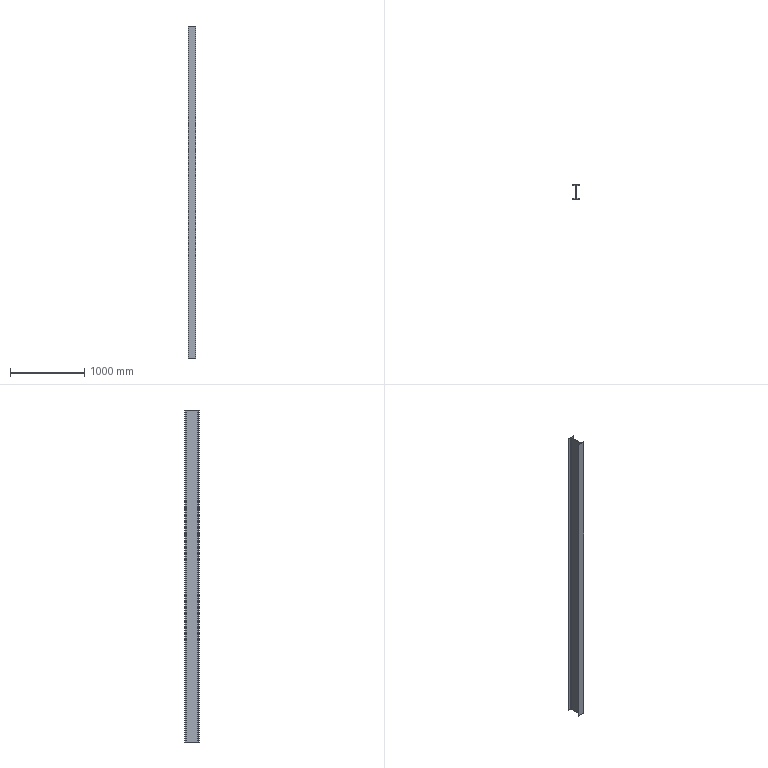Part | SolidWorks | features Extrusion 1, MoveFace 1 | 1 solid | 18 faces | box 100 x 200 x 4480 mm | volume 12833917 mm3 | plane 10 | cylinder 8 | commonest cylinder face diameters 9 x4 18 x4
STEP:
#1=CARTESIAN_POINT('',(314.405,123.017,-900.));
#2=VERTEX_POINT('',#1);
#3=CARTESIAN_POINT('',(321.925,131.894,-900.));
#4=VERTEX_POINT('',#3);
#5=CARTESIAN_POINT('',(323.405,123.017,-900.));
#6=DIRECTION('',(0.,0.,-1.));
#7=DIRECTION('',(1.,0.,0.));
#8=AXIS2_PLACEMENT_3D('',#5,#6,#7);
#9=CIRCLE('',#8,9.);
#10=EDGE_CURVE('',#2,#4,#9,.T.);
#11=ORIENTED_EDGE('',*,*,#10,.T.);
#12=CARTESIAN_POINT('',(321.925,131.894,3580.));
#13=VERTEX_POINT('',#12);
#14=CARTESIAN_POINT('',(321.925,131.894,3580.));
#15=DIRECTION('',(0.,0.,-1.));
#16=VECTOR('',#15,1000.);
#17=LINE('',#14,#16);
#18=EDGE_CURVE('',#13,#4,#17,.T.);
#19=ORIENTED_EDGE('',*,*,#18,.F.);
#20=CARTESIAN_POINT('',(314.405,123.017,3580.));
#21=VERTEX_POINT('',#20);
#22=CARTESIAN_POINT('',(323.405,123.017,3580.));
#23=DIRECTION('',(0.,0.,-1.));
#24=DIRECTION('',(1.,0.,0.));
#25=AXIS2_PLACEMENT_3D('',#22,#23,#24);
#26=CIRCLE('',#25,9.);
#27=EDGE_CURVE('',#21,#13,#26,.T.);
#28=ORIENTED_EDGE('',*,*,#27,.F.);
#29=CARTESIAN_POINT('',(314.405,123.017,3580.));
#30=DIRECTION('',(0.,0.,-1.));
#31=VECTOR('',#30,1000.);
#32=LINE('',#29,#31);
#33=EDGE_CURVE('',#21,#2,#32,.T.);
#34=ORIENTED_EDGE('',*,*,#33,.T.);
#35=EDGE_LOOP('',(#11,#19,#28,#34));
#36=FACE_OUTER_BOUND('',#35,.T.);
#37=CARTESIAN_POINT('',(323.405,123.017,3580.));
#38=DIRECTION('',(0.,0.,-1.));
#39=DIRECTION('',(-1.,0.,0.));
#40=AXIS2_PLACEMENT_3D('',#37,#38,#39);
#41=CYLINDRICAL_SURFACE('',#40,9.);
#42=ADVANCED_FACE('',(#36),#41,.F.);
#43=CARTESIAN_POINT('',(357.144,137.763,-900.));
#44=VERTEX_POINT('',#43);
#45=CARTESIAN_POINT('',(321.925,131.894,-900.));
#46=DIRECTION('',(0.9864,0.1644,0.));
#47=VECTOR('',#46,1000.);
#48=LINE('',#45,#47);
#49=EDGE_CURVE('',#4,#44,#48,.T.);
#50=ORIENTED_EDGE('',*,*,#49,.T.);
#51=CARTESIAN_POINT('',(357.144,137.763,3580.));
#52=VERTEX_POINT('',#51);
#53=CARTESIAN_POINT('',(357.144,137.763,3580.));
#54=DIRECTION('',(0.,0.,-1.));
#55=VECTOR('',#54,1000.);
#56=LINE('',#53,#55);
#57=EDGE_CURVE('',#52,#44,#56,.T.);
#58=ORIENTED_EDGE('',*,*,#57,.F.);
#59=CARTESIAN_POINT('',(321.925,131.894,3580.));
#60=DIRECTION('',(0.9864,0.1644,0.));
#61=VECTOR('',#60,1000.);
#62=LINE('',#59,#61);
#63=EDGE_CURVE('',#13,#52,#62,.T.);
#64=ORIENTED_EDGE('',*,*,#63,.F.);
#65=ORIENTED_EDGE('',*,*,#18,.T.);
#66=EDGE_LOOP('',(#50,#58,#64,#65));
#67=FACE_OUTER_BOUND('',#66,.T.);
#68=CARTESIAN_POINT('',(321.925,131.894,3580.));
#69=DIRECTION('',(-0.1644,0.9864,0.));
#70=DIRECTION('',(-0.9864,-0.1644,0.));
#71=AXIS2_PLACEMENT_3D('',#68,#69,#70);
#72=PLANE('',#71);
#73=ADVANCED_FACE('',(#67),#72,.F.);
#74=CARTESIAN_POINT('',(360.905,142.202,-900.));
#75=VERTEX_POINT('',#74);
#76=CARTESIAN_POINT('',(356.405,142.202,-900.));
#77=DIRECTION('',(0.,0.,1.));
#78=DIRECTION('',(1.,0.,0.));
#79=AXIS2_PLACEMENT_3D('',#76,#77,#78);
#80=CIRCLE('',#79,4.5);
#81=EDGE_CURVE('',#44,#75,#80,.T.);
#82=ORIENTED_EDGE('',*,*,#81,.T.);
#83=CARTESIAN_POINT('',(360.905,142.202,3580.));
#84=VERTEX_POINT('',#83);
#85=CARTESIAN_POINT('',(360.905,142.202,3580.));
#86=DIRECTION('',(0.,0.,-1.));
#87=VECTOR('',#86,1000.);
#88=LINE('',#85,#87);
#89=EDGE_CURVE('',#84,#75,#88,.T.);
#90=ORIENTED_EDGE('',*,*,#89,.F.);
#91=CARTESIAN_POINT('',(356.405,142.202,3580.));
#92=DIRECTION('',(0.,0.,1.));
#93=DIRECTION('',(1.,0.,0.));
#94=AXIS2_PLACEMENT_3D('',#91,#92,#93);
#95=CIRCLE('',#94,4.5);
#96=EDGE_CURVE('',#52,#84,#95,.T.);
#97=ORIENTED_EDGE('',*,*,#96,.F.);
#98=ORIENTED_EDGE('',*,*,#57,.T.);
#99=EDGE_LOOP('',(#82,#90,#97,#98));
#100=FACE_OUTER_BOUND('',#99,.T.);
#101=CARTESIAN_POINT('',(356.405,142.202,3580.));
#102=DIRECTION('',(0.,0.,-1.));
#103=DIRECTION('',(-1.,0.,0.));
#104=AXIS2_PLACEMENT_3D('',#101,#102,#103);
#105=CYLINDRICAL_SURFACE('',#104,4.5);
#106=ADVANCED_FACE('',(#100),#105,.T.);
#107=CARTESIAN_POINT('',(260.905,142.202,-900.));
#108=VERTEX_POINT('',#107);
#109=CARTESIAN_POINT('',(310.905,142.202,-900.));
#110=DIRECTION('',(-1.,0.,0.));
#111=VECTOR('',#110,1000.);
#112=LINE('',#109,#111);
#113=EDGE_CURVE('',#75,#108,#112,.T.);
#114=ORIENTED_EDGE('',*,*,#113,.T.);
#115=CARTESIAN_POINT('',(260.905,142.202,3580.));
#116=VERTEX_POINT('',#115);
#117=CARTESIAN_POINT('',(260.905,142.202,3580.));
#118=DIRECTION('',(0.,0.,-1.));
#119=VECTOR('',#118,1000.);
#120=LINE('',#117,#119);
#121=EDGE_CURVE('',#116,#108,#120,.T.);
#122=ORIENTED_EDGE('',*,*,#121,.F.);
#123=CARTESIAN_POINT('',(310.905,142.202,3580.));
#124=DIRECTION('',(-1.,0.,0.));
#125=VECTOR('',#124,1000.);
#126=LINE('',#123,#125);
#127=EDGE_CURVE('',#84,#116,#126,.T.);
#128=ORIENTED_EDGE('',*,*,#127,.F.);
#129=ORIENTED_EDGE('',*,*,#89,.T.);
#130=EDGE_LOOP('',(#114,#122,#128,#129));
#131=FACE_OUTER_BOUND('',#130,.T.);
#132=CARTESIAN_POINT('',(310.905,142.202,3580.));
#133=DIRECTION('',(0.,-1.,0.));
#134=DIRECTION('',(0.,0.,-1.));
#135=AXIS2_PLACEMENT_3D('',#132,#133,#134);
#136=PLANE('',#135);
#137=ADVANCED_FACE('',(#131),#136,.F.);
#138=CARTESIAN_POINT('',(264.665,137.763,-900.));
#139=VERTEX_POINT('',#138);
#140=CARTESIAN_POINT('',(265.405,142.202,-900.));
#141=DIRECTION('',(0.,0.,1.));
#142=DIRECTION('',(1.,0.,0.));
#143=AXIS2_PLACEMENT_3D('',#140,#141,#142);
#144=CIRCLE('',#143,4.5);
#145=EDGE_CURVE('',#108,#139,#144,.T.);
#146=ORIENTED_EDGE('',*,*,#145,.T.);
#147=CARTESIAN_POINT('',(264.665,137.763,3580.));
#148=VERTEX_POINT('',#147);
#149=CARTESIAN_POINT('',(264.665,137.763,3580.));
#150=DIRECTION('',(0.,0.,-1.));
#151=VECTOR('',#150,1000.);
#152=LINE('',#149,#151);
#153=EDGE_CURVE('',#148,#139,#152,.T.);
#154=ORIENTED_EDGE('',*,*,#153,.F.);
#155=CARTESIAN_POINT('',(265.405,142.202,3580.));
#156=DIRECTION('',(0.,0.,1.));
#157=DIRECTION('',(1.,0.,0.));
#158=AXIS2_PLACEMENT_3D('',#155,#156,#157);
#159=CIRCLE('',#158,4.5);
#160=EDGE_CURVE('',#116,#148,#159,.T.);
#161=ORIENTED_EDGE('',*,*,#160,.F.);
#162=ORIENTED_EDGE('',*,*,#121,.T.);
#163=EDGE_LOOP('',(#146,#154,#161,#162));
#164=FACE_OUTER_BOUND('',#163,.T.);
#165=CARTESIAN_POINT('',(265.405,142.202,3580.));
#166=DIRECTION('',(0.,0.,-1.));
#167=DIRECTION('',(-1.,0.,0.));
#168=AXIS2_PLACEMENT_3D('',#165,#166,#167);
#169=CYLINDRICAL_SURFACE('',#168,4.5);
#170=ADVANCED_FACE('',(#164),#169,.T.);
#171=CARTESIAN_POINT('',(299.884,131.894,-900.));
#172=VERTEX_POINT('',#171);
#173=CARTESIAN_POINT('',(299.884,131.894,-900.));
#174=DIRECTION('',(0.9864,-0.1644,0.));
#175=VECTOR('',#174,1000.);
#176=LINE('',#173,#175);
#177=EDGE_CURVE('',#139,#172,#176,.T.);
#178=ORIENTED_EDGE('',*,*,#177,.T.);
#179=CARTESIAN_POINT('',(299.884,131.894,3580.));
#180=VERTEX_POINT('',#179);
#181=CARTESIAN_POINT('',(299.884,131.894,3580.));
#182=DIRECTION('',(0.,0.,-1.));
#183=VECTOR('',#182,1000.);
#184=LINE('',#181,#183);
#185=EDGE_CURVE('',#180,#172,#184,.T.);
#186=ORIENTED_EDGE('',*,*,#185,.F.);
#187=CARTESIAN_POINT('',(299.884,131.894,3580.));
#188=DIRECTION('',(0.9864,-0.1644,0.));
#189=VECTOR('',#188,1000.);
#190=LINE('',#187,#189);
#191=EDGE_CURVE('',#148,#180,#190,.T.);
#192=ORIENTED_EDGE('',*,*,#191,.F.);
#193=ORIENTED_EDGE('',*,*,#153,.T.);
#194=EDGE_LOOP('',(#178,#186,#192,#193));
#195=FACE_OUTER_BOUND('',#194,.T.);
#196=CARTESIAN_POINT('',(299.884,131.894,3580.));
#197=DIRECTION('',(0.1644,0.9864,0.));
#198=DIRECTION('',(-0.9864,0.1644,0.));
#199=AXIS2_PLACEMENT_3D('',#196,#197,#198);
#200=PLANE('',#199);
#201=ADVANCED_FACE('',(#195),#200,.F.);
#202=CARTESIAN_POINT('',(307.405,123.017,-900.));
#203=VERTEX_POINT('',#202);
#204=CARTESIAN_POINT('',(298.405,123.017,-900.));
#205=DIRECTION('',(0.,0.,-1.));
#206=DIRECTION('',(1.,0.,0.));
#207=AXIS2_PLACEMENT_3D('',#204,#205,#206);
#208=CIRCLE('',#207,9.);
#209=EDGE_CURVE('',#172,#203,#208,.T.);
#210=ORIENTED_EDGE('',*,*,#209,.T.);
#211=CARTESIAN_POINT('',(307.405,123.017,3580.));
#212=VERTEX_POINT('',#211);
#213=CARTESIAN_POINT('',(307.405,123.017,3580.));
#214=DIRECTION('',(0.,0.,-1.));
#215=VECTOR('',#214,1000.);
#216=LINE('',#213,#215);
#217=EDGE_CURVE('',#212,#203,#216,.T.);
#218=ORIENTED_EDGE('',*,*,#217,.F.);
#219=CARTESIAN_POINT('',(298.405,123.017,3580.));
#220=DIRECTION('',(0.,0.,-1.));
#221=DIRECTION('',(1.,0.,0.));
#222=AXIS2_PLACEMENT_3D('',#219,#220,#221);
#223=CIRCLE('',#222,9.);
#224=EDGE_CURVE('',#180,#212,#223,.T.);
#225=ORIENTED_EDGE('',*,*,#224,.F.);
#226=ORIENTED_EDGE('',*,*,#185,.T.);
#227=EDGE_LOOP('',(#210,#218,#225,#226));
#228=FACE_OUTER_BOUND('',#227,.T.);
#229=CARTESIAN_POINT('',(298.405,123.017,3580.));
#230=DIRECTION('',(0.,0.,-1.));
#231=DIRECTION('',(-1.,0.,0.));
#232=AXIS2_PLACEMENT_3D('',#229,#230,#231);
#233=CYLINDRICAL_SURFACE('',#232,9.);
#234=ADVANCED_FACE('',(#228),#233,.F.);
#235=CARTESIAN_POINT('',(307.405,-38.614,-900.));
#236=VERTEX_POINT('',#235);
#237=CARTESIAN_POINT('',(307.405,42.202,-900.));
#238=DIRECTION('',(0.,-1.,0.));
#239=VECTOR('',#238,1000.);
#240=LINE('',#237,#239);
#241=EDGE_CURVE('',#203,#236,#240,.T.);
#242=ORIENTED_EDGE('',*,*,#241,.T.);
#243=CARTESIAN_POINT('',(307.405,-38.614,3580.));
#244=VERTEX_POINT('',#243);
#245=CARTESIAN_POINT('',(307.405,-38.614,3580.));
#246=DIRECTION('',(0.,0.,-1.));
#247=VECTOR('',#246,1000.);
#248=LINE('',#245,#247);
#249=EDGE_CURVE('',#244,#236,#248,.T.);
#250=ORIENTED_EDGE('',*,*,#249,.F.);
#251=CARTESIAN_POINT('',(307.405,42.202,3580.));
#252=DIRECTION('',(0.,-1.,0.));
#253=VECTOR('',#252,1000.);
#254=LINE('',#251,#253);
#255=EDGE_CURVE('',#212,#244,#254,.T.);
#256=ORIENTED_EDGE('',*,*,#255,.F.);
#257=ORIENTED_EDGE('',*,*,#217,.T.);
#258=EDGE_LOOP('',(#242,#250,#256,#257));
#259=FACE_OUTER_BOUND('',#258,.T.);
#260=CARTESIAN_POINT('',(307.405,42.202,3580.));
#261=DIRECTION('',(1.,0.,0.));
#262=DIRECTION('',(0.,0.,-1.));
#263=AXIS2_PLACEMENT_3D('',#260,#261,#262);
#264=PLANE('',#263);
#265=ADVANCED_FACE('',(#259),#264,.F.);
#266=CARTESIAN_POINT('',(299.884,-47.491,-900.));
#267=VERTEX_POINT('',#266);
#268=CARTESIAN_POINT('',(298.405,-38.614,-900.));
#269=DIRECTION('',(0.,0.,-1.));
#270=DIRECTION('',(1.,0.,0.));
#271=AXIS2_PLACEMENT_3D('',#268,#269,#270);
#272=CIRCLE('',#271,9.);
#273=EDGE_CURVE('',#236,#267,#272,.T.);
#274=ORIENTED_EDGE('',*,*,#273,.T.);
#275=CARTESIAN_POINT('',(299.884,-47.491,3580.));
#276=VERTEX_POINT('',#275);
#277=CARTESIAN_POINT('',(299.884,-47.491,3580.));
#278=DIRECTION('',(0.,0.,-1.));
#279=VECTOR('',#278,1000.);
#280=LINE('',#277,#279);
#281=EDGE_CURVE('',#276,#267,#280,.T.);
#282=ORIENTED_EDGE('',*,*,#281,.F.);
#283=CARTESIAN_POINT('',(298.405,-38.614,3580.));
#284=DIRECTION('',(0.,0.,-1.));
#285=DIRECTION('',(1.,0.,0.));
#286=AXIS2_PLACEMENT_3D('',#283,#284,#285);
#287=CIRCLE('',#286,9.);
#288=EDGE_CURVE('',#244,#276,#287,.T.);
#289=ORIENTED_EDGE('',*,*,#288,.F.);
#290=ORIENTED_EDGE('',*,*,#249,.T.);
#291=EDGE_LOOP('',(#274,#282,#289,#290));
#292=FACE_OUTER_BOUND('',#291,.T.);
#293=CARTESIAN_POINT('',(298.405,-38.614,3580.));
#294=DIRECTION('',(0.,0.,-1.));
#295=DIRECTION('',(-1.,0.,0.));
#296=AXIS2_PLACEMENT_3D('',#293,#294,#295);
#297=CYLINDRICAL_SURFACE('',#296,9.);
#298=ADVANCED_FACE('',(#292),#297,.F.);
#299=CARTESIAN_POINT('',(264.665,-53.36,-900.));
#300=VERTEX_POINT('',#299);
#301=CARTESIAN_POINT('',(299.884,-47.491,-900.));
#302=DIRECTION('',(-0.9864,-0.1644,0.));
#303=VECTOR('',#302,1000.);
#304=LINE('',#301,#303);
#305=EDGE_CURVE('',#267,#300,#304,.T.);
#306=ORIENTED_EDGE('',*,*,#305,.T.);
#307=CARTESIAN_POINT('',(264.665,-53.36,3580.));
#308=VERTEX_POINT('',#307);
#309=CARTESIAN_POINT('',(264.665,-53.36,3580.));
#310=DIRECTION('',(0.,0.,-1.));
#311=VECTOR('',#310,1000.);
#312=LINE('',#309,#311);
#313=EDGE_CURVE('',#308,#300,#312,.T.);
#314=ORIENTED_EDGE('',*,*,#313,.F.);
#315=CARTESIAN_POINT('',(299.884,-47.491,3580.));
#316=DIRECTION('',(-0.9864,-0.1644,0.));
#317=VECTOR('',#316,1000.);
#318=LINE('',#315,#317);
#319=EDGE_CURVE('',#276,#308,#318,.T.);
#320=ORIENTED_EDGE('',*,*,#319,.F.);
#321=ORIENTED_EDGE('',*,*,#281,.T.);
#322=EDGE_LOOP('',(#306,#314,#320,#321));
#323=FACE_OUTER_BOUND('',#322,.T.);
#324=CARTESIAN_POINT('',(299.884,-47.491,3580.));
#325=DIRECTION('',(0.1644,-0.9864,0.));
#326=DIRECTION('',(0.9864,0.1644,0.));
#327=AXIS2_PLACEMENT_3D('',#324,#325,#326);
#328=PLANE('',#327);
#329=ADVANCED_FACE('',(#323),#328,.F.);
#330=CARTESIAN_POINT('',(260.905,-57.798,-900.));
#331=VERTEX_POINT('',#330);
#332=CARTESIAN_POINT('',(265.405,-57.798,-900.));
#333=DIRECTION('',(0.,0.,1.));
#334=DIRECTION('',(1.,0.,0.));
#335=AXIS2_PLACEMENT_3D('',#332,#333,#334);
#336=CIRCLE('',#335,4.5);
#337=EDGE_CURVE('',#300,#331,#336,.T.);
#338=ORIENTED_EDGE('',*,*,#337,.T.);
#339=CARTESIAN_POINT('',(260.905,-57.798,3580.));
#340=VERTEX_POINT('',#339);
#341=CARTESIAN_POINT('',(260.905,-57.798,3580.));
#342=DIRECTION('',(0.,0.,-1.));
#343=VECTOR('',#342,1000.);
#344=LINE('',#341,#343);
#345=EDGE_CURVE('',#340,#331,#344,.T.);
#346=ORIENTED_EDGE('',*,*,#345,.F.);
#347=CARTESIAN_POINT('',(265.405,-57.798,3580.));
#348=DIRECTION('',(0.,0.,1.));
#349=DIRECTION('',(1.,0.,0.));
#350=AXIS2_PLACEMENT_3D('',#347,#348,#349);
#351=CIRCLE('',#350,4.5);
#352=EDGE_CURVE('',#308,#340,#351,.T.);
#353=ORIENTED_EDGE('',*,*,#352,.F.);
#354=ORIENTED_EDGE('',*,*,#313,.T.);
#355=EDGE_LOOP('',(#338,#346,#353,#354));
#356=FACE_OUTER_BOUND('',#355,.T.);
#357=CARTESIAN_POINT('',(265.405,-57.798,3580.));
#358=DIRECTION('',(0.,0.,-1.));
#359=DIRECTION('',(-1.,0.,0.));
#360=AXIS2_PLACEMENT_3D('',#357,#358,#359);
#361=CYLINDRICAL_SURFACE('',#360,4.5);
#362=ADVANCED_FACE('',(#356),#361,.T.);
#363=CARTESIAN_POINT('',(360.905,-57.798,-900.));
#364=VERTEX_POINT('',#363);
#365=CARTESIAN_POINT('',(310.905,-57.798,-900.));
#366=DIRECTION('',(1.,0.,0.));
#367=VECTOR('',#366,1000.);
#368=LINE('',#365,#367);
#369=EDGE_CURVE('',#331,#364,#368,.T.);
#370=ORIENTED_EDGE('',*,*,#369,.T.);
#371=CARTESIAN_POINT('',(360.905,-57.798,3580.));
#372=VERTEX_POINT('',#371);
#373=CARTESIAN_POINT('',(360.905,-57.798,3580.));
#374=DIRECTION('',(0.,0.,-1.));
#375=VECTOR('',#374,1000.);
#376=LINE('',#373,#375);
#377=EDGE_CURVE('',#372,#364,#376,.T.);
#378=ORIENTED_EDGE('',*,*,#377,.F.);
#379=CARTESIAN_POINT('',(310.905,-57.798,3580.));
#380=DIRECTION('',(1.,0.,0.));
#381=VECTOR('',#380,1000.);
#382=LINE('',#379,#381);
#383=EDGE_CURVE('',#340,#372,#382,.T.);
#384=ORIENTED_EDGE('',*,*,#383,.F.);
#385=ORIENTED_EDGE('',*,*,#345,.T.);
#386=EDGE_LOOP('',(#370,#378,#384,#385));
#387=FACE_OUTER_BOUND('',#386,.T.);
#388=CARTESIAN_POINT('',(310.905,-57.798,3580.));
#389=DIRECTION('',(0.,1.,0.));
#390=DIRECTION('',(0.,0.,1.));
#391=AXIS2_PLACEMENT_3D('',#388,#389,#390);
#392=PLANE('',#391);
#393=ADVANCED_FACE('',(#387),#392,.F.);
#394=CARTESIAN_POINT('',(357.144,-53.36,-900.));
#395=VERTEX_POINT('',#394);
#396=CARTESIAN_POINT('',(356.405,-57.798,-900.));
#397=DIRECTION('',(0.,0.,1.));
#398=DIRECTION('',(1.,0.,0.));
#399=AXIS2_PLACEMENT_3D('',#396,#397,#398);
#400=CIRCLE('',#399,4.5);
#401=EDGE_CURVE('',#364,#395,#400,.T.);
#402=ORIENTED_EDGE('',*,*,#401,.T.);
#403=CARTESIAN_POINT('',(357.144,-53.36,3580.));
#404=VERTEX_POINT('',#403);
#405=CARTESIAN_POINT('',(357.144,-53.36,3580.));
#406=DIRECTION('',(0.,0.,-1.));
#407=VECTOR('',#406,1000.);
#408=LINE('',#405,#407);
#409=EDGE_CURVE('',#404,#395,#408,.T.);
#410=ORIENTED_EDGE('',*,*,#409,.F.);
#411=CARTESIAN_POINT('',(356.405,-57.798,3580.));
#412=DIRECTION('',(0.,0.,1.));
#413=DIRECTION('',(1.,0.,0.));
#414=AXIS2_PLACEMENT_3D('',#411,#412,#413);
#415=CIRCLE('',#414,4.5);
#416=EDGE_CURVE('',#372,#404,#415,.T.);
#417=ORIENTED_EDGE('',*,*,#416,.F.);
#418=ORIENTED_EDGE('',*,*,#377,.T.);
#419=EDGE_LOOP('',(#402,#410,#417,#418));
#420=FACE_OUTER_BOUND('',#419,.T.);
#421=CARTESIAN_POINT('',(356.405,-57.798,3580.));
#422=DIRECTION('',(0.,0.,-1.));
#423=DIRECTION('',(-1.,0.,0.));
#424=AXIS2_PLACEMENT_3D('',#421,#422,#423);
#425=CYLINDRICAL_SURFACE('',#424,4.5);
#426=ADVANCED_FACE('',(#420),#425,.T.);
#427=CARTESIAN_POINT('',(321.925,-47.491,-900.));
#428=VERTEX_POINT('',#427);
#429=CARTESIAN_POINT('',(321.925,-47.491,-900.));
#430=DIRECTION('',(-0.9864,0.1644,0.));
#431=VECTOR('',#430,1000.);
#432=LINE('',#429,#431);
#433=EDGE_CURVE('',#395,#428,#432,.T.);
#434=ORIENTED_EDGE('',*,*,#433,.T.);
#435=CARTESIAN_POINT('',(321.925,-47.491,3580.));
#436=VERTEX_POINT('',#435);
#437=CARTESIAN_POINT('',(321.925,-47.491,3580.));
#438=DIRECTION('',(0.,0.,-1.));
#439=VECTOR('',#438,1000.);
#440=LINE('',#437,#439);
#441=EDGE_CURVE('',#436,#428,#440,.T.);
#442=ORIENTED_EDGE('',*,*,#441,.F.);
#443=CARTESIAN_POINT('',(321.925,-47.491,3580.));
#444=DIRECTION('',(-0.9864,0.1644,0.));
#445=VECTOR('',#444,1000.);
#446=LINE('',#443,#445);
#447=EDGE_CURVE('',#404,#436,#446,.T.);
#448=ORIENTED_EDGE('',*,*,#447,.F.);
#449=ORIENTED_EDGE('',*,*,#409,.T.);
#450=EDGE_LOOP('',(#434,#442,#448,#449));
#451=FACE_OUTER_BOUND('',#450,.T.);
#452=CARTESIAN_POINT('',(321.925,-47.491,3580.));
#453=DIRECTION('',(-0.1644,-0.9864,0.));
#454=DIRECTION('',(0.9864,-0.1644,0.));
#455=AXIS2_PLACEMENT_3D('',#452,#453,#454);
#456=PLANE('',#455);
#457=ADVANCED_FACE('',(#451),#456,.F.);
#458=CARTESIAN_POINT('',(314.405,-38.614,-900.));
#459=VERTEX_POINT('',#458);
#460=CARTESIAN_POINT('',(323.405,-38.614,-900.));
#461=DIRECTION('',(0.,0.,-1.));
#462=DIRECTION('',(1.,0.,0.));
#463=AXIS2_PLACEMENT_3D('',#460,#461,#462);
#464=CIRCLE('',#463,9.);
#465=EDGE_CURVE('',#428,#459,#464,.T.);
#466=ORIENTED_EDGE('',*,*,#465,.T.);
#467=CARTESIAN_POINT('',(314.405,-38.614,3580.));
#468=VERTEX_POINT('',#467);
#469=CARTESIAN_POINT('',(314.405,-38.614,3580.));
#470=DIRECTION('',(0.,0.,-1.));
#471=VECTOR('',#470,1000.);
#472=LINE('',#469,#471);
#473=EDGE_CURVE('',#468,#459,#472,.T.);
#474=ORIENTED_EDGE('',*,*,#473,.F.);
#475=CARTESIAN_POINT('',(323.405,-38.614,3580.));
#476=DIRECTION('',(0.,0.,-1.));
#477=DIRECTION('',(1.,0.,0.));
#478=AXIS2_PLACEMENT_3D('',#475,#476,#477);
#479=CIRCLE('',#478,9.);
#480=EDGE_CURVE('',#436,#468,#479,.T.);
#481=ORIENTED_EDGE('',*,*,#480,.F.);
#482=ORIENTED_EDGE('',*,*,#441,.T.);
#483=EDGE_LOOP('',(#466,#474,#481,#482));
#484=FACE_OUTER_BOUND('',#483,.T.);
#485=CARTESIAN_POINT('',(323.405,-38.614,3580.));
#486=DIRECTION('',(0.,0.,-1.));
#487=DIRECTION('',(-1.,0.,0.));
#488=AXIS2_PLACEMENT_3D('',#485,#486,#487);
#489=CYLINDRICAL_SURFACE('',#488,9.);
#490=ADVANCED_FACE('',(#484),#489,.F.);
#491=CARTESIAN_POINT('',(314.405,42.202,-900.));
#492=DIRECTION('',(0.,1.,0.));
#493=VECTOR('',#492,1000.);
#494=LINE('',#491,#493);
#495=EDGE_CURVE('',#459,#2,#494,.T.);
#496=ORIENTED_EDGE('',*,*,#495,.T.);
#497=ORIENTED_EDGE('',*,*,#33,.F.);
#498=CARTESIAN_POINT('',(314.405,42.202,3580.));
#499=DIRECTION('',(0.,1.,0.));
#500=VECTOR('',#499,1000.);
#501=LINE('',#498,#500);
#502=EDGE_CURVE('',#468,#21,#501,.T.);
#503=ORIENTED_EDGE('',*,*,#502,.F.);
#504=ORIENTED_EDGE('',*,*,#473,.T.);
#505=EDGE_LOOP('',(#496,#497,#503,#504));
#506=FACE_OUTER_BOUND('',#505,.T.);
#507=CARTESIAN_POINT('',(314.405,42.202,3580.));
#508=DIRECTION('',(-1.,0.,0.));
#509=DIRECTION('',(0.,0.,1.));
#510=AXIS2_PLACEMENT_3D('',#507,#508,#509);
#511=PLANE('',#510);
#512=ADVANCED_FACE('',(#506),#511,.F.);
#513=ORIENTED_EDGE('',*,*,#27,.T.);
#514=ORIENTED_EDGE('',*,*,#63,.T.);
#515=ORIENTED_EDGE('',*,*,#96,.T.);
#516=ORIENTED_EDGE('',*,*,#127,.T.);
#517=ORIENTED_EDGE('',*,*,#160,.T.);
#518=ORIENTED_EDGE('',*,*,#191,.T.);
#519=ORIENTED_EDGE('',*,*,#224,.T.);
#520=ORIENTED_EDGE('',*,*,#255,.T.);
#521=ORIENTED_EDGE('',*,*,#288,.T.);
#522=ORIENTED_EDGE('',*,*,#319,.T.);
#523=ORIENTED_EDGE('',*,*,#352,.T.);
#524=ORIENTED_EDGE('',*,*,#383,.T.);
#525=ORIENTED_EDGE('',*,*,#416,.T.);
#526=ORIENTED_EDGE('',*,*,#447,.T.);
#527=ORIENTED_EDGE('',*,*,#480,.T.);
#528=ORIENTED_EDGE('',*,*,#502,.T.);
#529=EDGE_LOOP('',(#513,#514,#515,#516,#517,#518,#519,#520,#521,#522,#523,#524,#525,#526,#527,#528));
#530=FACE_OUTER_BOUND('',#529,.T.);
#531=CARTESIAN_POINT('',(323.405,123.017,3580.));
#532=DIRECTION('',(0.,0.,1.));
#533=DIRECTION('',(1.,0.,0.));
#534=AXIS2_PLACEMENT_3D('',#531,#532,#533);
#535=PLANE('',#534);
#536=ADVANCED_FACE('',(#530),#535,.T.);
#537=ORIENTED_EDGE('',*,*,#10,.F.);
#538=ORIENTED_EDGE('',*,*,#495,.F.);
#539=ORIENTED_EDGE('',*,*,#465,.F.);
#540=ORIENTED_EDGE('',*,*,#433,.F.);
#541=ORIENTED_EDGE('',*,*,#401,.F.);
#542=ORIENTED_EDGE('',*,*,#369,.F.);
#543=ORIENTED_EDGE('',*,*,#337,.F.);
#544=ORIENTED_EDGE('',*,*,#305,.F.);
#545=ORIENTED_EDGE('',*,*,#273,.F.);
#546=ORIENTED_EDGE('',*,*,#241,.F.);
#547=ORIENTED_EDGE('',*,*,#209,.F.);
#548=ORIENTED_EDGE('',*,*,#177,.F.);
#549=ORIENTED_EDGE('',*,*,#145,.F.);
#550=ORIENTED_EDGE('',*,*,#113,.F.);
#551=ORIENTED_EDGE('',*,*,#81,.F.);
#552=ORIENTED_EDGE('',*,*,#49,.F.);
#553=EDGE_LOOP('',(#537,#538,#539,#540,#541,#542,#543,#544,#545,#546,#547,#548,#549,#550,#551,#552));
#554=FACE_OUTER_BOUND('',#553,.T.);
#555=CARTESIAN_POINT('',(323.405,123.017,-900.));
#556=DIRECTION('',(0.,0.,1.));
#557=DIRECTION('',(1.,0.,0.));
#558=AXIS2_PLACEMENT_3D('',#555,#556,#557);
#559=PLANE('',#558);
#560=ADVANCED_FACE('',(#554),#559,.F.);
#561=CLOSED_SHELL('',(#42,#73,#106,#137,#170,#201,#234,#265,#298,#329,#362,#393,#426,#457,#490,#512,#536,#560));
#562=MANIFOLD_SOLID_BREP('',#561);
#563=CARTESIAN_POINT('',(0.,0.,0.));
#564=DIRECTION('',(0.,0.,1.));
#565=DIRECTION('',(1.,0.,0.));
#566=AXIS2_PLACEMENT_3D('',#563,#564,#565);
#567=(LENGTH_UNIT()NAMED_UNIT(*)SI_UNIT(.MILLI.,.METRE.));
#568=UNCERTAINTY_MEASURE_WITH_UNIT(LENGTH_MEASURE(0.00001),#567,'','');
#569=(NAMED_UNIT(*)PLANE_ANGLE_UNIT()SI_UNIT($,.RADIAN.));
#570=(NAMED_UNIT(*)SI_UNIT($,.STERADIAN.)SOLID_ANGLE_UNIT());
#571=(GEOMETRIC_REPRESENTATION_CONTEXT(3)GLOBAL_UNCERTAINTY_ASSIGNED_CONTEXT((#568))GLOBAL_UNIT_ASSIGNED_CONTEXT((#567,#569,#570))REPRESENTATION_CONTEXT('',''));
#572=ADVANCED_BREP_SHAPE_REPRESENTATION('',(#562,#566),#571);